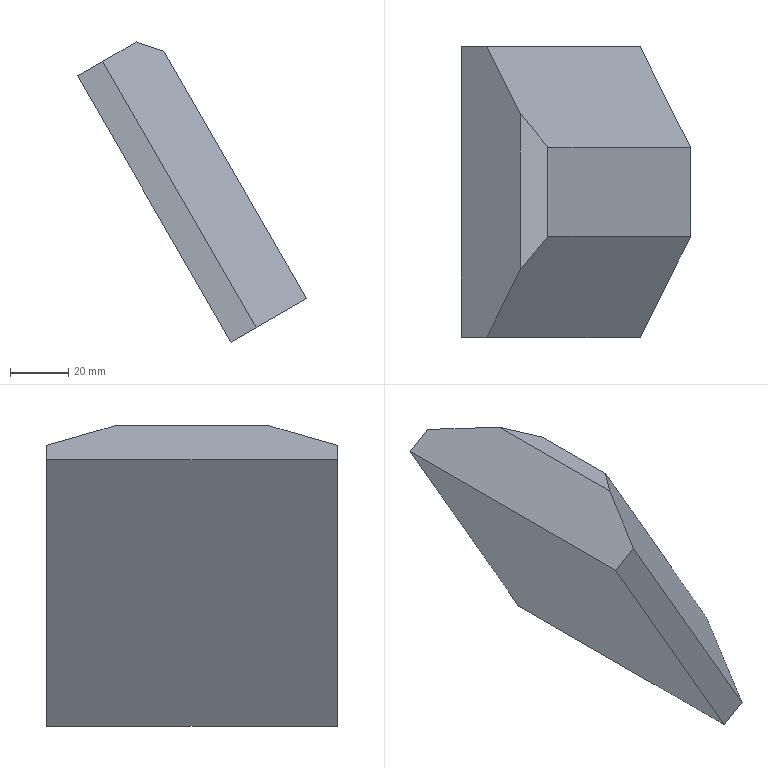Part | NX | features solid 2 | 1 solid | 9 faces | box 78.81 x 100 x 103.2 mm | volume 242824 mm3 | plane 9
STEP:
#1=CARTESIAN_POINT('',(-16.342,709.641,290.003));
#2=VERTEX_POINT('',#1);
#3=CARTESIAN_POINT('',(-16.342,740.359,290.003));
#4=VERTEX_POINT('',#3);
#5=CARTESIAN_POINT('',(-16.342,675.,290.003));
#6=DIRECTION('',(0.,1.,0.));
#7=VECTOR('',#6,1000.);
#8=LINE('',#5,#7);
#9=EDGE_CURVE('',#2,#4,#8,.T.);
#10=ORIENTED_EDGE('',*,*,#9,.T.);
#11=CARTESIAN_POINT('',(-25.817,751.803,293.2));
#12=VERTEX_POINT('',#11);
#13=CARTESIAN_POINT('',(20.61,695.728,277.535));
#14=DIRECTION('',(0.6235,-0.753,-0.2104));
#15=VECTOR('',#14,1000.);
#16=LINE('',#13,#15);
#17=EDGE_CURVE('',#4,#12,#16,.F.);
#18=ORIENTED_EDGE('',*,*,#17,.T.);
#19=CARTESIAN_POINT('',(-25.817,698.197,293.2));
#20=VERTEX_POINT('',#19);
#21=CARTESIAN_POINT('',(-25.817,675.,293.2));
#22=DIRECTION('',(0.,1.,0.));
#23=VECTOR('',#22,1000.);
#24=LINE('',#21,#23);
#25=EDGE_CURVE('',#20,#12,#24,.T.);
#26=ORIENTED_EDGE('',*,*,#25,.F.);
#27=CARTESIAN_POINT('',(-26.189,697.748,293.325));
#28=DIRECTION('',(0.6235,0.753,-0.2104));
#29=VECTOR('',#28,1000.);
#30=LINE('',#27,#29);
#31=EDGE_CURVE('',#20,#2,#30,.T.);
#32=ORIENTED_EDGE('',*,*,#31,.T.);
#33=EDGE_LOOP('',(#10,#18,#26,#32));
#34=FACE_BOUND('',#33,.T.);
#35=CARTESIAN_POINT('',(-16.342,675.,290.003));
#36=DIRECTION('',(-0.3197,0.,-0.9475));
#37=DIRECTION('',(-0.9475,0.,0.3197));
#38=AXIS2_PLACEMENT_3D('',#35,#36,#37);
#39=PLANE('',#38);
#40=ADVANCED_FACE('',(#34),#39,.F.);
#41=ORIENTED_EDGE('',*,*,#25,.T.);
#42=CARTESIAN_POINT('',(-37.416,775.,286.504));
#43=VERTEX_POINT('',#42);
#44=CARTESIAN_POINT('',(-20.095,740.359,296.504));
#45=DIRECTION('',(0.433,-0.866,0.25));
#46=VECTOR('',#45,1000.);
#47=LINE('',#44,#46);
#48=EDGE_CURVE('',#12,#43,#47,.F.);
#49=ORIENTED_EDGE('',*,*,#48,.T.);
#50=CARTESIAN_POINT('',(-46.076,775.,281.504));
#51=VERTEX_POINT('',#50);
#52=CARTESIAN_POINT('',(-25.817,775.,293.2));
#53=DIRECTION('',(-0.866,0.,-0.5));
#54=VECTOR('',#53,1000.);
#55=LINE('',#52,#54);
#56=EDGE_CURVE('',#43,#51,#55,.T.);
#57=ORIENTED_EDGE('',*,*,#56,.T.);
#58=CARTESIAN_POINT('',(-46.076,675.,281.504));
#59=VERTEX_POINT('',#58);
#60=CARTESIAN_POINT('',(-46.076,675.,281.504));
#61=DIRECTION('',(0.,1.,0.));
#62=VECTOR('',#61,1000.);
#63=LINE('',#60,#62);
#64=EDGE_CURVE('',#59,#51,#63,.T.);
#65=ORIENTED_EDGE('',*,*,#64,.F.);
#66=CARTESIAN_POINT('',(-37.416,675.,286.504));
#67=VERTEX_POINT('',#66);
#68=CARTESIAN_POINT('',(-25.817,675.,293.2));
#69=DIRECTION('',(-0.866,0.,-0.5));
#70=VECTOR('',#69,1000.);
#71=LINE('',#68,#70);
#72=EDGE_CURVE('',#67,#59,#71,.T.);
#73=ORIENTED_EDGE('',*,*,#72,.F.);
#74=CARTESIAN_POINT('',(-37.416,675.,286.504));
#75=DIRECTION('',(0.433,0.866,0.25));
#76=VECTOR('',#75,1000.);
#77=LINE('',#74,#76);
#78=EDGE_CURVE('',#67,#20,#77,.T.);
#79=ORIENTED_EDGE('',*,*,#78,.T.);
#80=EDGE_LOOP('',(#41,#49,#57,#65,#73,#79));
#81=FACE_BOUND('',#80,.T.);
#82=CARTESIAN_POINT('',(-25.817,675.,293.2));
#83=DIRECTION('',(0.5,0.,-0.866));
#84=DIRECTION('',(-0.866,0.,-0.5));
#85=AXIS2_PLACEMENT_3D('',#82,#83,#84);
#86=PLANE('',#85);
#87=ADVANCED_FACE('',(#81),#86,.F.);
#88=CARTESIAN_POINT('',(6.753,775.,190.));
#89=VERTEX_POINT('',#88);
#90=CARTESIAN_POINT('',(-46.076,775.,281.504));
#91=DIRECTION('',(0.5,0.,-0.866));
#92=VECTOR('',#91,1000.);
#93=LINE('',#90,#92);
#94=EDGE_CURVE('',#51,#89,#93,.T.);
#95=ORIENTED_EDGE('',*,*,#94,.T.);
#96=CARTESIAN_POINT('',(6.753,675.,190.));
#97=VERTEX_POINT('',#96);
#98=CARTESIAN_POINT('',(6.753,675.,190.));
#99=DIRECTION('',(0.,1.,0.));
#100=VECTOR('',#99,1000.);
#101=LINE('',#98,#100);
#102=EDGE_CURVE('',#97,#89,#101,.T.);
#103=ORIENTED_EDGE('',*,*,#102,.F.);
#104=CARTESIAN_POINT('',(-46.076,675.,281.504));
#105=DIRECTION('',(0.5,0.,-0.866));
#106=VECTOR('',#105,1000.);
#107=LINE('',#104,#106);
#108=EDGE_CURVE('',#59,#97,#107,.T.);
#109=ORIENTED_EDGE('',*,*,#108,.F.);
#110=ORIENTED_EDGE('',*,*,#64,.T.);
#111=EDGE_LOOP('',(#95,#103,#109,#110));
#112=FACE_BOUND('',#111,.T.);
#113=CARTESIAN_POINT('',(-46.076,675.,281.504));
#114=DIRECTION('',(0.866,0.,0.5));
#115=DIRECTION('',(0.5,0.,-0.866));
#116=AXIS2_PLACEMENT_3D('',#113,#114,#115);
#117=PLANE('',#116);
#118=ADVANCED_FACE('',(#112),#117,.F.);
#119=CARTESIAN_POINT('',(15.414,775.,195.));
#120=VERTEX_POINT('',#119);
#121=CARTESIAN_POINT('',(6.753,775.,190.));
#122=DIRECTION('',(0.866,0.,0.5));
#123=VECTOR('',#122,1000.);
#124=LINE('',#121,#123);
#125=EDGE_CURVE('',#89,#120,#124,.T.);
#126=ORIENTED_EDGE('',*,*,#125,.T.);
#127=CARTESIAN_POINT('',(32.734,740.359,205.));
#128=VERTEX_POINT('',#127);
#129=CARTESIAN_POINT('',(32.734,740.359,205.));
#130=DIRECTION('',(-0.433,0.866,-0.25));
#131=VECTOR('',#130,1000.);
#132=LINE('',#129,#131);
#133=EDGE_CURVE('',#120,#128,#132,.F.);
#134=ORIENTED_EDGE('',*,*,#133,.T.);
#135=CARTESIAN_POINT('',(32.734,709.641,205.));
#136=VERTEX_POINT('',#135);
#137=CARTESIAN_POINT('',(32.734,675.,205.));
#138=DIRECTION('',(0.,1.,0.));
#139=VECTOR('',#138,1000.);
#140=LINE('',#137,#139);
#141=EDGE_CURVE('',#136,#128,#140,.T.);
#142=ORIENTED_EDGE('',*,*,#141,.F.);
#143=CARTESIAN_POINT('',(15.414,675.,195.));
#144=VERTEX_POINT('',#143);
#145=CARTESIAN_POINT('',(15.414,675.,195.));
#146=DIRECTION('',(-0.433,-0.866,-0.25));
#147=VECTOR('',#146,1000.);
#148=LINE('',#145,#147);
#149=EDGE_CURVE('',#136,#144,#148,.T.);
#150=ORIENTED_EDGE('',*,*,#149,.T.);
#151=CARTESIAN_POINT('',(6.753,675.,190.));
#152=DIRECTION('',(0.866,0.,0.5));
#153=VECTOR('',#152,1000.);
#154=LINE('',#151,#153);
#155=EDGE_CURVE('',#97,#144,#154,.T.);
#156=ORIENTED_EDGE('',*,*,#155,.F.);
#157=ORIENTED_EDGE('',*,*,#102,.T.);
#158=EDGE_LOOP('',(#126,#134,#142,#150,#156,#157));
#159=FACE_BOUND('',#158,.T.);
#160=CARTESIAN_POINT('',(6.753,675.,190.));
#161=DIRECTION('',(-0.5,0.,0.866));
#162=DIRECTION('',(0.866,0.,0.5));
#163=AXIS2_PLACEMENT_3D('',#160,#161,#162);
#164=PLANE('',#163);
#165=ADVANCED_FACE('',(#159),#164,.F.);
#166=ORIENTED_EDGE('',*,*,#141,.T.);
#167=CARTESIAN_POINT('',(43.658,740.359,186.08));
#168=DIRECTION('',(-0.5,0.,0.866));
#169=VECTOR('',#168,1000.);
#170=LINE('',#167,#169);
#171=EDGE_CURVE('',#128,#4,#170,.T.);
#172=ORIENTED_EDGE('',*,*,#171,.T.);
#173=ORIENTED_EDGE('',*,*,#9,.F.);
#174=CARTESIAN_POINT('',(32.734,709.641,205.));
#175=DIRECTION('',(0.5,0.,-0.866));
#176=VECTOR('',#175,1000.);
#177=LINE('',#174,#176);
#178=EDGE_CURVE('',#2,#136,#177,.T.);
#179=ORIENTED_EDGE('',*,*,#178,.T.);
#180=EDGE_LOOP('',(#166,#172,#173,#179));
#181=FACE_BOUND('',#180,.T.);
#182=CARTESIAN_POINT('',(43.658,675.,186.08));
#183=DIRECTION('',(-0.866,0.,-0.5));
#184=DIRECTION('',(-0.5,0.,0.866));
#185=AXIS2_PLACEMENT_3D('',#182,#183,#184);
#186=PLANE('',#185);
#187=ADVANCED_FACE('',(#181),#186,.F.);
#188=ORIENTED_EDGE('',*,*,#155,.T.);
#189=CARTESIAN_POINT('',(-33.663,675.,280.003));
#190=DIRECTION('',(-0.5,0.,0.866));
#191=VECTOR('',#190,1000.);
#192=LINE('',#189,#191);
#193=EDGE_CURVE('',#144,#67,#192,.T.);
#194=ORIENTED_EDGE('',*,*,#193,.T.);
#195=ORIENTED_EDGE('',*,*,#72,.T.);
#196=ORIENTED_EDGE('',*,*,#108,.T.);
#197=EDGE_LOOP('',(#188,#194,#195,#196));
#198=FACE_BOUND('',#197,.T.);
#199=CARTESIAN_POINT('',(-8.657,675.,250.049));
#200=DIRECTION('',(0.,-1.,0.));
#201=DIRECTION('',(0.,0.,-1.));
#202=AXIS2_PLACEMENT_3D('',#199,#200,#201);
#203=PLANE('',#202);
#204=ADVANCED_FACE('',(#198),#203,.T.);
#205=ORIENTED_EDGE('',*,*,#56,.F.);
#206=CARTESIAN_POINT('',(-14.441,775.,246.71));
#207=DIRECTION('',(0.5,0.,-0.866));
#208=VECTOR('',#207,1000.);
#209=LINE('',#206,#208);
#210=EDGE_CURVE('',#43,#120,#209,.T.);
#211=ORIENTED_EDGE('',*,*,#210,.T.);
#212=ORIENTED_EDGE('',*,*,#125,.F.);
#213=ORIENTED_EDGE('',*,*,#94,.F.);
#214=EDGE_LOOP('',(#205,#211,#212,#213));
#215=FACE_BOUND('',#214,.T.);
#216=CARTESIAN_POINT('',(-8.657,775.,250.049));
#217=DIRECTION('',(0.,-1.,0.));
#218=DIRECTION('',(0.,0.,-1.));
#219=AXIS2_PLACEMENT_3D('',#216,#217,#218);
#220=PLANE('',#219);
#221=ADVANCED_FACE('',(#215),#220,.F.);
#222=ORIENTED_EDGE('',*,*,#149,.F.);
#223=ORIENTED_EDGE('',*,*,#178,.F.);
#224=ORIENTED_EDGE('',*,*,#31,.F.);
#225=ORIENTED_EDGE('',*,*,#78,.F.);
#226=ORIENTED_EDGE('',*,*,#193,.F.);
#227=EDGE_LOOP('',(#222,#223,#224,#225,#226));
#228=FACE_BOUND('',#227,.T.);
#229=CARTESIAN_POINT('',(-14.441,675.,246.71));
#230=DIRECTION('',(0.75,-0.5,0.433));
#231=DIRECTION('',(0.5547,0.8321,0.));
#232=AXIS2_PLACEMENT_3D('',#229,#230,#231);
#233=PLANE('',#232);
#234=ADVANCED_FACE('',(#228),#233,.T.);
#235=ORIENTED_EDGE('',*,*,#133,.F.);
#236=ORIENTED_EDGE('',*,*,#210,.F.);
#237=ORIENTED_EDGE('',*,*,#48,.F.);
#238=ORIENTED_EDGE('',*,*,#17,.F.);
#239=ORIENTED_EDGE('',*,*,#171,.F.);
#240=EDGE_LOOP('',(#235,#236,#237,#238,#239));
#241=FACE_BOUND('',#240,.T.);
#242=CARTESIAN_POINT('',(43.658,740.359,186.08));
#243=DIRECTION('',(-0.75,-0.5,-0.433));
#244=DIRECTION('',(0.5547,-0.8321,0.));
#245=AXIS2_PLACEMENT_3D('',#242,#243,#244);
#246=PLANE('',#245);
#247=ADVANCED_FACE('',(#241),#246,.F.);
#248=CLOSED_SHELL('',(#40,#87,#118,#165,#187,#204,#221,#234,#247));
#249=MANIFOLD_SOLID_BREP('',#248);
#250=(LENGTH_UNIT()NAMED_UNIT(*)SI_UNIT(.MILLI.,.METRE.));
#251=UNCERTAINTY_MEASURE_WITH_UNIT(LENGTH_MEASURE(0.00001),#250,'','');
#252=(NAMED_UNIT(*)PLANE_ANGLE_UNIT()SI_UNIT($,.RADIAN.));
#253=(NAMED_UNIT(*)SI_UNIT($,.STERADIAN.)SOLID_ANGLE_UNIT());
#254=(GEOMETRIC_REPRESENTATION_CONTEXT(3)GLOBAL_UNCERTAINTY_ASSIGNED_CONTEXT((#251))GLOBAL_UNIT_ASSIGNED_CONTEXT((#250,#252,#253))REPRESENTATION_CONTEXT('',''));
#255=ADVANCED_BREP_SHAPE_REPRESENTATION('',(#249),#254);